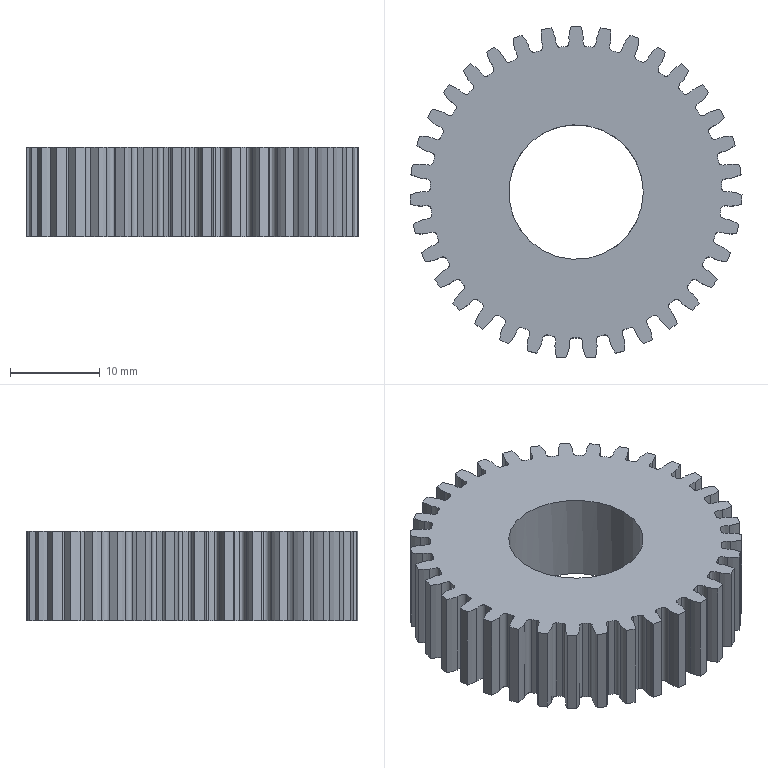Part | NX | features BREP 35, META 35, DATUM_CSYS 2, CYLINDER 1, EXTRUDE 1, FSET 1, SKETCH 1 | 1 solid | 213 faces | box 37 x 37 x 10 mm | volume 7712 mm3 | spline 175 | cylinder 36 | plane 2 | commonest cylinder face diameters 32.5 x35 15 x1